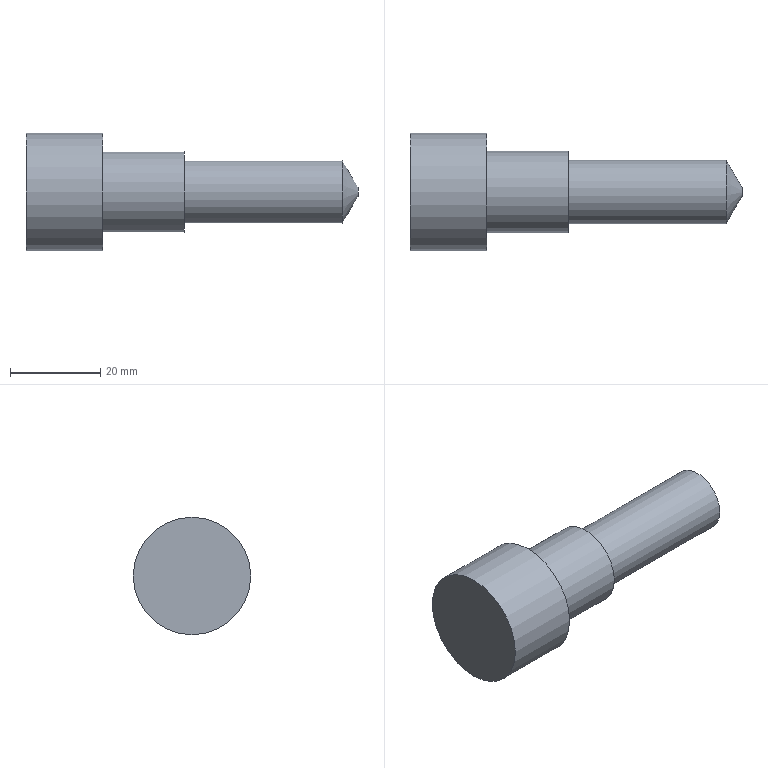Part | STEP file | solid 64 | 1 solid | 8 faces | box 73.5 x 26 x 26 mm | volume 19201 mm3 | plane 4 | cylinder 3 | cone 1 | commonest cylinder face diameters 14 x1 18 x1 26 x1